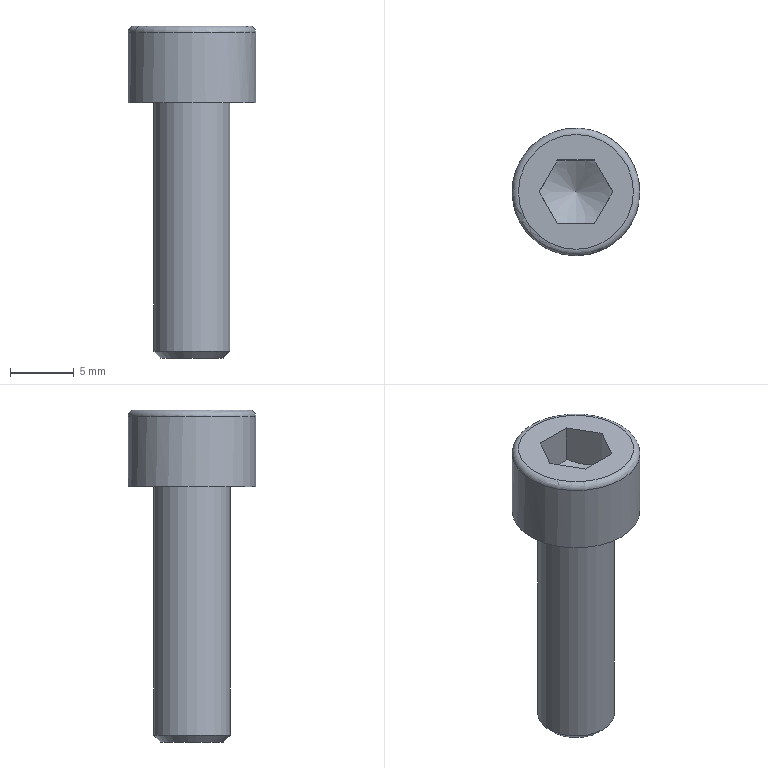Part | STEP file | 1_19 | 1 solid | 14 faces | box 10 x 10 x 26 mm | volume 953.385 mm3 | plane 9 | cylinder 2 | cone 2 | torus 1 | commonest cylinder face diameters 6 x1 10 x1
STEP:
#1=CARTESIAN_POINT('',(0.,0.,0.));
#2=DIRECTION('',(0.,0.,1.));
#3=DIRECTION('',(1.,0.,0.));
#4=AXIS2_PLACEMENT_3D('',#1,#2,#3);
#5=CARTESIAN_POINT('',(0.,-5.,0.));
#6=VERTEX_POINT('',#5);
#7=CARTESIAN_POINT('',(0.,0.,0.));
#8=DIRECTION('',(0.,0.,1.));
#9=DIRECTION('',(1.,0.,0.));
#10=AXIS2_PLACEMENT_3D('',#7,#8,#9);
#11=CIRCLE('',#10,5.);
#12=CARTESIAN_POINT('',(0.,0.,2.75));
#13=DIRECTION('',(0.,0.,1.));
#14=DIRECTION('',(0.,-1.,0.));
#15=AXIS2_PLACEMENT_3D('',#12,#13,#14);
#16=CYLINDRICAL_SURFACE('',#15,5.);
#17=CARTESIAN_POINT('',(-4.712,-2.75));
#18=DIRECTION('',(1.,0.));
#19=VECTOR('',#18,1.);
#20=LINE('',#17,#19);
#21=(GEOMETRIC_REPRESENTATION_CONTEXT(2)PARAMETRIC_REPRESENTATION_CONTEXT()REPRESENTATION_CONTEXT('',''));
#22=DEFINITIONAL_REPRESENTATION('',(#20),#21);
#23=PCURVE('',#16,#22);
#24=CARTESIAN_POINT('',(0.,2.5,0.));
#25=DIRECTION('',(0.,0.,-1.));
#26=DIRECTION('',(-1.,0.,0.));
#27=AXIS2_PLACEMENT_3D('',#24,#25,#26);
#28=PLANE('',#27);
#29=CARTESIAN_POINT('',(-5.,-2.5));
#30=CARTESIAN_POINT('',(-5.,6.16));
#31=CARTESIAN_POINT('',(2.5,1.83));
#32=CARTESIAN_POINT('',(10.,-2.5));
#33=CARTESIAN_POINT('',(2.5,-6.83));
#34=CARTESIAN_POINT('',(-5.,-11.16));
#35=CARTESIAN_POINT('',(-5.,-2.5));
#36=(BOUNDED_CURVE()B_SPLINE_CURVE(2,(#29,#30,#31,#32,#33,#34,#35),.UNSPECIFIED.,.T.,.F.)B_SPLINE_CURVE_WITH_KNOTS((1,2,2,2,2,1),(-2.094,0.,2.094,4.189,6.283,8.378),.UNSPECIFIED.)CURVE()GEOMETRIC_REPRESENTATION_ITEM()RATIONAL_B_SPLINE_CURVE((1.,0.5,1.,0.5,1.,0.5,1.))REPRESENTATION_ITEM(''));
#37=(GEOMETRIC_REPRESENTATION_CONTEXT(2)PARAMETRIC_REPRESENTATION_CONTEXT()REPRESENTATION_CONTEXT('',''));
#38=DEFINITIONAL_REPRESENTATION('',(#36),#37);
#39=PCURVE('',#28,#38);
#40=SURFACE_CURVE('',#11,(#23,#39),.PCURVE_S1.);
#41=EDGE_CURVE('',#6,#6,#40,.T.);
#42=ORIENTED_EDGE('',*,*,#41,.T.);
#43=CARTESIAN_POINT('',(0.,-5.,5.5));
#44=VERTEX_POINT('',#43);
#45=CARTESIAN_POINT('',(0.,-5.,0.));
#46=CARTESIAN_POINT('',(0.,-5.,5.5));
#47=B_SPLINE_CURVE_WITH_KNOTS('',1,(#45,#46),.UNSPECIFIED.,.F.,.F.,(2,2),(-2.75,2.75),.PIECEWISE_BEZIER_KNOTS.);
#48=CARTESIAN_POINT('',(6.283,0.));
#49=DIRECTION('',(0.,1.));
#50=VECTOR('',#49,1.);
#51=LINE('',#48,#50);
#52=(GEOMETRIC_REPRESENTATION_CONTEXT(2)PARAMETRIC_REPRESENTATION_CONTEXT()REPRESENTATION_CONTEXT('',''));
#53=DEFINITIONAL_REPRESENTATION('',(#51),#52);
#54=PCURVE('',#16,#53);
#55=CARTESIAN_POINT('',(0.,0.));
#56=DIRECTION('',(0.,1.));
#57=VECTOR('',#56,1.);
#58=LINE('',#55,#57);
#59=(GEOMETRIC_REPRESENTATION_CONTEXT(2)PARAMETRIC_REPRESENTATION_CONTEXT()REPRESENTATION_CONTEXT('',''));
#60=DEFINITIONAL_REPRESENTATION('',(#58),#59);
#61=PCURVE('',#16,#60);
#62=SEAM_CURVE('',#47,(#54,#61),.PCURVE_S1.);
#63=EDGE_CURVE('',#6,#44,#62,.T.);
#64=ORIENTED_EDGE('',*,*,#63,.T.);
#65=CARTESIAN_POINT('',(5.,0.,5.5));
#66=VERTEX_POINT('',#65);
#67=CARTESIAN_POINT('',(0.,0.,5.5));
#68=DIRECTION('',(0.,0.,1.));
#69=DIRECTION('',(1.,0.,0.));
#70=AXIS2_PLACEMENT_3D('',#67,#68,#69);
#71=CIRCLE('',#70,5.);
#72=CARTESIAN_POINT('',(1.571,2.75));
#73=DIRECTION('',(1.,0.));
#74=VECTOR('',#73,1.);
#75=LINE('',#72,#74);
#76=(GEOMETRIC_REPRESENTATION_CONTEXT(2)PARAMETRIC_REPRESENTATION_CONTEXT()REPRESENTATION_CONTEXT('',''));
#77=DEFINITIONAL_REPRESENTATION('',(#75),#76);
#78=PCURVE('',#16,#77);
#79=CARTESIAN_POINT('',(0.,0.,5.5));
#80=DIRECTION('',(0.,0.,-1.));
#81=DIRECTION('',(-1.,0.,0.));
#82=AXIS2_PLACEMENT_3D('',#79,#80,#81);
#83=TOROIDAL_SURFACE('',#82,4.5,0.5);
#84=CARTESIAN_POINT('',(9.425,6.283));
#85=DIRECTION('',(-1.,0.));
#86=VECTOR('',#85,1.);
#87=LINE('',#84,#86);
#88=(GEOMETRIC_REPRESENTATION_CONTEXT(2)PARAMETRIC_REPRESENTATION_CONTEXT()REPRESENTATION_CONTEXT('',''));
#89=DEFINITIONAL_REPRESENTATION('',(#87),#88);
#90=PCURVE('',#83,#89);
#91=SURFACE_CURVE('',#71,(#78,#90),.PCURVE_S1.);
#92=EDGE_CURVE('',#66,#44,#91,.T.);
#93=ORIENTED_EDGE('',*,*,#92,.F.);
#94=CARTESIAN_POINT('',(0.,0.,5.5));
#95=DIRECTION('',(0.,0.,1.));
#96=DIRECTION('',(1.,0.,0.));
#97=AXIS2_PLACEMENT_3D('',#94,#95,#96);
#98=CIRCLE('',#97,5.);
#99=CARTESIAN_POINT('',(-4.712,2.75));
#100=DIRECTION('',(1.,0.));
#101=VECTOR('',#100,1.);
#102=LINE('',#99,#101);
#103=(GEOMETRIC_REPRESENTATION_CONTEXT(2)PARAMETRIC_REPRESENTATION_CONTEXT()REPRESENTATION_CONTEXT('',''));
#104=DEFINITIONAL_REPRESENTATION('',(#102),#103);
#105=PCURVE('',#16,#104);
#106=CARTESIAN_POINT('',(15.708,6.283));
#107=DIRECTION('',(-1.,0.));
#108=VECTOR('',#107,1.);
#109=LINE('',#106,#108);
#110=(GEOMETRIC_REPRESENTATION_CONTEXT(2)PARAMETRIC_REPRESENTATION_CONTEXT()REPRESENTATION_CONTEXT('',''));
#111=DEFINITIONAL_REPRESENTATION('',(#109),#110);
#112=PCURVE('',#83,#111);
#113=SURFACE_CURVE('',#98,(#105,#112),.PCURVE_S1.);
#114=EDGE_CURVE('',#44,#66,#113,.T.);
#115=ORIENTED_EDGE('',*,*,#114,.F.);
#116=ORIENTED_EDGE('',*,*,#63,.F.);
#117=EDGE_LOOP('',(#42,#64,#93,#115,#116));
#118=FACE_BOUND('',#117,.T.);
#119=ADVANCED_FACE('',(#118),#16,.T.);
#120=ORIENTED_EDGE('',*,*,#92,.T.);
#121=CARTESIAN_POINT('',(0.,-4.5,6.));
#122=VERTEX_POINT('',#121);
#123=CARTESIAN_POINT('',(0.,-4.5,6.));
#124=CARTESIAN_POINT('',(0.,-4.634,6.));
#125=CARTESIAN_POINT('',(0.,-4.764,5.957));
#126=CARTESIAN_POINT('',(0.,-4.876,5.876));
#127=CARTESIAN_POINT('',(0.,-4.957,5.764));
#128=CARTESIAN_POINT('',(0.,-5.,5.634));
#129=CARTESIAN_POINT('',(0.,-5.,5.5));
#130=(BOUNDED_CURVE()B_SPLINE_CURVE(6,(#123,#124,#125,#126,#127,#128,#129),.UNSPECIFIED.,.F.,.F.)B_SPLINE_CURVE_WITH_KNOTS((7,7),(-1.571,0.),.PIECEWISE_BEZIER_KNOTS.)CURVE()GEOMETRIC_REPRESENTATION_ITEM()RATIONAL_B_SPLINE_CURVE((1.031,1.01,0.9979,0.994,0.9979,1.01,1.031))REPRESENTATION_ITEM(''));
#131=CARTESIAN_POINT('',(4.712,6.283));
#132=DIRECTION('',(0.,1.));
#133=VECTOR('',#132,1.);
#134=LINE('',#131,#133);
#135=(GEOMETRIC_REPRESENTATION_CONTEXT(2)PARAMETRIC_REPRESENTATION_CONTEXT()REPRESENTATION_CONTEXT('',''));
#136=DEFINITIONAL_REPRESENTATION('',(#134),#135);
#137=PCURVE('',#83,#136);
#138=CARTESIAN_POINT('',(10.996,6.283));
#139=DIRECTION('',(0.,1.));
#140=VECTOR('',#139,1.);
#141=LINE('',#138,#140);
#142=(GEOMETRIC_REPRESENTATION_CONTEXT(2)PARAMETRIC_REPRESENTATION_CONTEXT()REPRESENTATION_CONTEXT('',''));
#143=DEFINITIONAL_REPRESENTATION('',(#141),#142);
#144=PCURVE('',#83,#143);
#145=SEAM_CURVE('',#130,(#137,#144),.PCURVE_S1.);
#146=EDGE_CURVE('',#122,#44,#145,.T.);
#147=ORIENTED_EDGE('',*,*,#146,.F.);
#148=CARTESIAN_POINT('',(0.,4.5,6.));
#149=VERTEX_POINT('',#148);
#150=CARTESIAN_POINT('',(0.,0.,6.));
#151=DIRECTION('',(0.,0.,-1.));
#152=DIRECTION('',(1.,0.,0.));
#153=AXIS2_PLACEMENT_3D('',#150,#151,#152);
#154=CIRCLE('',#153,4.5);
#155=CARTESIAN_POINT('',(3.142,4.712));
#156=DIRECTION('',(1.,0.));
#157=VECTOR('',#156,1.);
#158=LINE('',#155,#157);
#159=(GEOMETRIC_REPRESENTATION_CONTEXT(2)PARAMETRIC_REPRESENTATION_CONTEXT()REPRESENTATION_CONTEXT('',''));
#160=DEFINITIONAL_REPRESENTATION('',(#158),#159);
#161=PCURVE('',#83,#160);
#162=CARTESIAN_POINT('',(0.,2.25,6.));
#163=DIRECTION('',(0.,0.,1.));
#164=DIRECTION('',(1.,0.,0.));
#165=AXIS2_PLACEMENT_3D('',#162,#163,#164);
#166=PLANE('',#165);
#167=CARTESIAN_POINT('',(4.5,-2.25));
#168=CARTESIAN_POINT('',(4.5,-10.044));
#169=CARTESIAN_POINT('',(-2.25,-6.147));
#170=CARTESIAN_POINT('',(-9.,-2.25));
#171=CARTESIAN_POINT('',(-2.25,1.647));
#172=CARTESIAN_POINT('',(4.5,5.544));
#173=CARTESIAN_POINT('',(4.5,-2.25));
#174=(BOUNDED_CURVE()B_SPLINE_CURVE(2,(#167,#168,#169,#170,#171,#172,#173),.UNSPECIFIED.,.T.,.F.)B_SPLINE_CURVE_WITH_KNOTS((1,2,2,2,2,1),(-2.094,0.,2.094,4.189,6.283,8.378),.UNSPECIFIED.)CURVE()GEOMETRIC_REPRESENTATION_ITEM()RATIONAL_B_SPLINE_CURVE((1.,0.5,1.,0.5,1.,0.5,1.))REPRESENTATION_ITEM(''));
#175=(GEOMETRIC_REPRESENTATION_CONTEXT(2)PARAMETRIC_REPRESENTATION_CONTEXT()REPRESENTATION_CONTEXT('',''));
#176=DEFINITIONAL_REPRESENTATION('',(#174),#175);
#177=PCURVE('',#166,#176);
#178=SURFACE_CURVE('',#154,(#161,#177),.PCURVE_S1.);
#179=EDGE_CURVE('',#122,#149,#178,.T.);
#180=ORIENTED_EDGE('',*,*,#179,.T.);
#181=CARTESIAN_POINT('',(0.,0.,6.));
#182=DIRECTION('',(0.,0.,-1.));
#183=DIRECTION('',(1.,0.,0.));
#184=AXIS2_PLACEMENT_3D('',#181,#182,#183);
#185=CIRCLE('',#184,4.5);
#186=CARTESIAN_POINT('',(3.142,4.712));
#187=DIRECTION('',(1.,0.));
#188=VECTOR('',#187,1.);
#189=LINE('',#186,#188);
#190=(GEOMETRIC_REPRESENTATION_CONTEXT(2)PARAMETRIC_REPRESENTATION_CONTEXT()REPRESENTATION_CONTEXT('',''));
#191=DEFINITIONAL_REPRESENTATION('',(#189),#190);
#192=PCURVE('',#83,#191);
#193=CARTESIAN_POINT('',(4.5,-2.25));
#194=CARTESIAN_POINT('',(4.5,-10.044));
#195=CARTESIAN_POINT('',(-2.25,-6.147));
#196=CARTESIAN_POINT('',(-9.,-2.25));
#197=CARTESIAN_POINT('',(-2.25,1.647));
#198=CARTESIAN_POINT('',(4.5,5.544));
#199=CARTESIAN_POINT('',(4.5,-2.25));
#200=(BOUNDED_CURVE()B_SPLINE_CURVE(2,(#193,#194,#195,#196,#197,#198,#199),.UNSPECIFIED.,.T.,.F.)B_SPLINE_CURVE_WITH_KNOTS((1,2,2,2,2,1),(-2.094,0.,2.094,4.189,6.283,8.378),.UNSPECIFIED.)CURVE()GEOMETRIC_REPRESENTATION_ITEM()RATIONAL_B_SPLINE_CURVE((1.,0.5,1.,0.5,1.,0.5,1.))REPRESENTATION_ITEM(''));
#201=(GEOMETRIC_REPRESENTATION_CONTEXT(2)PARAMETRIC_REPRESENTATION_CONTEXT()REPRESENTATION_CONTEXT('',''));
#202=DEFINITIONAL_REPRESENTATION('',(#200),#201);
#203=PCURVE('',#166,#202);
#204=SURFACE_CURVE('',#185,(#192,#203),.PCURVE_S1.);
#205=EDGE_CURVE('',#149,#122,#204,.T.);
#206=ORIENTED_EDGE('',*,*,#205,.T.);
#207=ORIENTED_EDGE('',*,*,#146,.T.);
#208=ORIENTED_EDGE('',*,*,#114,.T.);
#209=EDGE_LOOP('',(#120,#147,#180,#206,#207,#208));
#210=FACE_BOUND('',#209,.T.);
#211=ADVANCED_FACE('',(#210),#83,.T.);
#212=ORIENTED_EDGE('',*,*,#41,.F.);
#213=EDGE_LOOP('',(#212));
#214=FACE_BOUND('',#213,.T.);
#215=CARTESIAN_POINT('',(0.,-3.,0.));
#216=VERTEX_POINT('',#215);
#217=CARTESIAN_POINT('',(0.,0.,0.));
#218=DIRECTION('',(0.,0.,1.));
#219=DIRECTION('',(0.,1.,0.));
#220=AXIS2_PLACEMENT_3D('',#217,#218,#219);
#221=CIRCLE('',#220,3.);
#222=CARTESIAN_POINT('',(0.,0.5));
#223=CARTESIAN_POINT('',(5.196,0.5));
#224=CARTESIAN_POINT('',(2.598,-4.));
#225=CARTESIAN_POINT('',(0.,-8.5));
#226=CARTESIAN_POINT('',(-2.598,-4.));
#227=CARTESIAN_POINT('',(-5.196,0.5));
#228=CARTESIAN_POINT('',(0.,0.5));
#229=(BOUNDED_CURVE()B_SPLINE_CURVE(2,(#222,#223,#224,#225,#226,#227,#228),.UNSPECIFIED.,.T.,.F.)B_SPLINE_CURVE_WITH_KNOTS((1,2,2,2,2,1),(-2.094,0.,2.094,4.189,6.283,8.378),.UNSPECIFIED.)CURVE()GEOMETRIC_REPRESENTATION_ITEM()RATIONAL_B_SPLINE_CURVE((1.,0.5,1.,0.5,1.,0.5,1.))REPRESENTATION_ITEM(''));
#230=(GEOMETRIC_REPRESENTATION_CONTEXT(2)PARAMETRIC_REPRESENTATION_CONTEXT()REPRESENTATION_CONTEXT('',''));
#231=DEFINITIONAL_REPRESENTATION('',(#229),#230);
#232=PCURVE('',#28,#231);
#233=CARTESIAN_POINT('',(0.,0.,-9.229));
#234=DIRECTION('',(0.,0.,1.));
#235=DIRECTION('',(0.,-1.,0.));
#236=AXIS2_PLACEMENT_3D('',#233,#234,#235);
#237=CYLINDRICAL_SURFACE('',#236,3.);
#238=CARTESIAN_POINT('',(-3.142,9.229));
#239=DIRECTION('',(1.,0.));
#240=VECTOR('',#239,1.);
#241=LINE('',#238,#240);
#242=(GEOMETRIC_REPRESENTATION_CONTEXT(2)PARAMETRIC_REPRESENTATION_CONTEXT()REPRESENTATION_CONTEXT('',''));
#243=DEFINITIONAL_REPRESENTATION('',(#241),#242);
#244=PCURVE('',#237,#243);
#245=SURFACE_CURVE('',#221,(#232,#244),.PCURVE_S1.);
#246=EDGE_CURVE('',#216,#216,#245,.T.);
#247=ORIENTED_EDGE('',*,*,#246,.T.);
#248=EDGE_LOOP('',(#247));
#249=FACE_BOUND('',#248,.T.);
#250=ADVANCED_FACE('',(#214,#249),#28,.T.);
#251=ORIENTED_EDGE('',*,*,#205,.F.);
#252=ORIENTED_EDGE('',*,*,#179,.F.);
#253=EDGE_LOOP('',(#251,#252));
#254=FACE_BOUND('',#253,.T.);
#255=CARTESIAN_POINT('',(-1.443,-2.5,6.));
#256=VERTEX_POINT('',#255);
#257=CARTESIAN_POINT('',(-2.887,0.,6.));
#258=VERTEX_POINT('',#257);
#259=CARTESIAN_POINT('',(-1.443,-2.5,6.));
#260=DIRECTION('',(-0.5,0.866,0.));
#261=VECTOR('',#260,1.);
#262=LINE('',#259,#261);
#263=CARTESIAN_POINT('',(-1.443,-4.75));
#264=DIRECTION('',(-0.5,0.866));
#265=VECTOR('',#264,1.);
#266=LINE('',#263,#265);
#267=(GEOMETRIC_REPRESENTATION_CONTEXT(2)PARAMETRIC_REPRESENTATION_CONTEXT()REPRESENTATION_CONTEXT('',''));
#268=DEFINITIONAL_REPRESENTATION('',(#266),#267);
#269=PCURVE('',#166,#268);
#270=CARTESIAN_POINT('',(-2.887,0.,6.));
#271=DIRECTION('',(-0.866,-0.5,0.));
#272=DIRECTION('',(0.,0.,1.));
#273=AXIS2_PLACEMENT_3D('',#270,#271,#272);
#274=PLANE('',#273);
#275=CARTESIAN_POINT('',(0.,-2.887));
#276=DIRECTION('',(0.,1.));
#277=VECTOR('',#276,1.);
#278=LINE('',#275,#277);
#279=(GEOMETRIC_REPRESENTATION_CONTEXT(2)PARAMETRIC_REPRESENTATION_CONTEXT()REPRESENTATION_CONTEXT('',''));
#280=DEFINITIONAL_REPRESENTATION('',(#278),#279);
#281=PCURVE('',#274,#280);
#282=SURFACE_CURVE('',#262,(#269,#281),.PCURVE_S1.);
#283=EDGE_CURVE('',#256,#258,#282,.T.);
#284=ORIENTED_EDGE('',*,*,#283,.T.);
#285=CARTESIAN_POINT('',(-1.443,2.5,6.));
#286=VERTEX_POINT('',#285);
#287=CARTESIAN_POINT('',(-2.887,0.,6.));
#288=DIRECTION('',(0.5,0.866,0.));
#289=VECTOR('',#288,1.);
#290=LINE('',#287,#289);
#291=CARTESIAN_POINT('',(-2.887,-2.25));
#292=DIRECTION('',(0.5,0.866));
#293=VECTOR('',#292,1.);
#294=LINE('',#291,#293);
#295=(GEOMETRIC_REPRESENTATION_CONTEXT(2)PARAMETRIC_REPRESENTATION_CONTEXT()REPRESENTATION_CONTEXT('',''));
#296=DEFINITIONAL_REPRESENTATION('',(#294),#295);
#297=PCURVE('',#166,#296);
#298=CARTESIAN_POINT('',(-1.443,2.5,6.));
#299=DIRECTION('',(-0.866,0.5,0.));
#300=DIRECTION('',(0.,0.,1.));
#301=AXIS2_PLACEMENT_3D('',#298,#299,#300);
#302=PLANE('',#301);
#303=CARTESIAN_POINT('',(0.,-2.887));
#304=DIRECTION('',(0.,1.));
#305=VECTOR('',#304,1.);
#306=LINE('',#303,#305);
#307=(GEOMETRIC_REPRESENTATION_CONTEXT(2)PARAMETRIC_REPRESENTATION_CONTEXT()REPRESENTATION_CONTEXT('',''));
#308=DEFINITIONAL_REPRESENTATION('',(#306),#307);
#309=PCURVE('',#302,#308);
#310=SURFACE_CURVE('',#290,(#297,#309),.PCURVE_S1.);
#311=EDGE_CURVE('',#258,#286,#310,.T.);
#312=ORIENTED_EDGE('',*,*,#311,.T.);
#313=CARTESIAN_POINT('',(1.443,2.5,6.));
#314=VERTEX_POINT('',#313);
#315=CARTESIAN_POINT('',(-1.443,2.5,6.));
#316=DIRECTION('',(1.,0.,0.));
#317=VECTOR('',#316,1.);
#318=LINE('',#315,#317);
#319=CARTESIAN_POINT('',(-1.443,0.25));
#320=DIRECTION('',(1.,0.));
#321=VECTOR('',#320,1.);
#322=LINE('',#319,#321);
#323=(GEOMETRIC_REPRESENTATION_CONTEXT(2)PARAMETRIC_REPRESENTATION_CONTEXT()REPRESENTATION_CONTEXT('',''));
#324=DEFINITIONAL_REPRESENTATION('',(#322),#323);
#325=PCURVE('',#166,#324);
#326=CARTESIAN_POINT('',(1.443,2.5,6.));
#327=DIRECTION('',(0.,1.,0.));
#328=DIRECTION('',(0.,0.,1.));
#329=AXIS2_PLACEMENT_3D('',#326,#327,#328);
#330=PLANE('',#329);
#331=CARTESIAN_POINT('',(0.,-2.887));
#332=DIRECTION('',(0.,1.));
#333=VECTOR('',#332,1.);
#334=LINE('',#331,#333);
#335=(GEOMETRIC_REPRESENTATION_CONTEXT(2)PARAMETRIC_REPRESENTATION_CONTEXT()REPRESENTATION_CONTEXT('',''));
#336=DEFINITIONAL_REPRESENTATION('',(#334),#335);
#337=PCURVE('',#330,#336);
#338=SURFACE_CURVE('',#318,(#325,#337),.PCURVE_S1.);
#339=EDGE_CURVE('',#286,#314,#338,.T.);
#340=ORIENTED_EDGE('',*,*,#339,.T.);
#341=CARTESIAN_POINT('',(2.887,0.,6.));
#342=VERTEX_POINT('',#341);
#343=CARTESIAN_POINT('',(1.443,2.5,6.));
#344=DIRECTION('',(0.5,-0.866,0.));
#345=VECTOR('',#344,1.);
#346=LINE('',#343,#345);
#347=CARTESIAN_POINT('',(1.443,0.25));
#348=DIRECTION('',(0.5,-0.866));
#349=VECTOR('',#348,1.);
#350=LINE('',#347,#349);
#351=(GEOMETRIC_REPRESENTATION_CONTEXT(2)PARAMETRIC_REPRESENTATION_CONTEXT()REPRESENTATION_CONTEXT('',''));
#352=DEFINITIONAL_REPRESENTATION('',(#350),#351);
#353=PCURVE('',#166,#352);
#354=CARTESIAN_POINT('',(2.887,0.,6.));
#355=DIRECTION('',(0.866,0.5,0.));
#356=DIRECTION('',(0.,0.,-1.));
#357=AXIS2_PLACEMENT_3D('',#354,#355,#356);
#358=PLANE('',#357);
#359=CARTESIAN_POINT('',(0.,2.887));
#360=DIRECTION('',(0.,-1.));
#361=VECTOR('',#360,1.);
#362=LINE('',#359,#361);
#363=(GEOMETRIC_REPRESENTATION_CONTEXT(2)PARAMETRIC_REPRESENTATION_CONTEXT()REPRESENTATION_CONTEXT('',''));
#364=DEFINITIONAL_REPRESENTATION('',(#362),#363);
#365=PCURVE('',#358,#364);
#366=SURFACE_CURVE('',#346,(#353,#365),.PCURVE_S1.);
#367=EDGE_CURVE('',#314,#342,#366,.T.);
#368=ORIENTED_EDGE('',*,*,#367,.T.);
#369=CARTESIAN_POINT('',(1.443,-2.5,6.));
#370=VERTEX_POINT('',#369);
#371=CARTESIAN_POINT('',(2.887,0.,6.));
#372=DIRECTION('',(-0.5,-0.866,0.));
#373=VECTOR('',#372,1.);
#374=LINE('',#371,#373);
#375=CARTESIAN_POINT('',(2.887,-2.25));
#376=DIRECTION('',(-0.5,-0.866));
#377=VECTOR('',#376,1.);
#378=LINE('',#375,#377);
#379=(GEOMETRIC_REPRESENTATION_CONTEXT(2)PARAMETRIC_REPRESENTATION_CONTEXT()REPRESENTATION_CONTEXT('',''));
#380=DEFINITIONAL_REPRESENTATION('',(#378),#379);
#381=PCURVE('',#166,#380);
#382=CARTESIAN_POINT('',(1.443,-2.5,6.));
#383=DIRECTION('',(0.866,-0.5,0.));
#384=DIRECTION('',(0.,0.,-1.));
#385=AXIS2_PLACEMENT_3D('',#382,#383,#384);
#386=PLANE('',#385);
#387=CARTESIAN_POINT('',(0.,2.887));
#388=DIRECTION('',(0.,-1.));
#389=VECTOR('',#388,1.);
#390=LINE('',#387,#389);
#391=(GEOMETRIC_REPRESENTATION_CONTEXT(2)PARAMETRIC_REPRESENTATION_CONTEXT()REPRESENTATION_CONTEXT('',''));
#392=DEFINITIONAL_REPRESENTATION('',(#390),#391);
#393=PCURVE('',#386,#392);
#394=SURFACE_CURVE('',#374,(#381,#393),.PCURVE_S1.);
#395=EDGE_CURVE('',#342,#370,#394,.T.);
#396=ORIENTED_EDGE('',*,*,#395,.T.);
#397=CARTESIAN_POINT('',(1.443,-2.5,6.));
#398=DIRECTION('',(-1.,0.,0.));
#399=VECTOR('',#398,1.);
#400=LINE('',#397,#399);
#401=CARTESIAN_POINT('',(1.443,-4.75));
#402=DIRECTION('',(-1.,0.));
#403=VECTOR('',#402,1.);
#404=LINE('',#401,#403);
#405=(GEOMETRIC_REPRESENTATION_CONTEXT(2)PARAMETRIC_REPRESENTATION_CONTEXT()REPRESENTATION_CONTEXT('',''));
#406=DEFINITIONAL_REPRESENTATION('',(#404),#405);
#407=PCURVE('',#166,#406);
#408=CARTESIAN_POINT('',(-1.443,-2.5,6.));
#409=DIRECTION('',(0.,-1.,0.));
#410=DIRECTION('',(0.,0.,-1.));
#411=AXIS2_PLACEMENT_3D('',#408,#409,#410);
#412=PLANE('',#411);
#413=CARTESIAN_POINT('',(0.,2.887));
#414=DIRECTION('',(0.,-1.));
#415=VECTOR('',#414,1.);
#416=LINE('',#413,#415);
#417=(GEOMETRIC_REPRESENTATION_CONTEXT(2)PARAMETRIC_REPRESENTATION_CONTEXT()REPRESENTATION_CONTEXT('',''));
#418=DEFINITIONAL_REPRESENTATION('',(#416),#417);
#419=PCURVE('',#412,#418);
#420=SURFACE_CURVE('',#400,(#407,#419),.PCURVE_S1.);
#421=EDGE_CURVE('',#370,#256,#420,.T.);
#422=ORIENTED_EDGE('',*,*,#421,.T.);
#423=EDGE_LOOP('',(#284,#312,#340,#368,#396,#422));
#424=FACE_BOUND('',#423,.T.);
#425=ADVANCED_FACE('',(#254,#424),#166,.T.);
#426=CARTESIAN_POINT('',(0.,-3.,-19.459));
#427=VERTEX_POINT('',#426);
#428=CARTESIAN_POINT('',(0.,0.,-19.459));
#429=DIRECTION('',(0.,0.,1.));
#430=DIRECTION('',(1.,0.,0.));
#431=AXIS2_PLACEMENT_3D('',#428,#429,#430);
#432=CIRCLE('',#431,3.);
#433=CARTESIAN_POINT('',(-4.712,-10.229));
#434=DIRECTION('',(1.,0.));
#435=VECTOR('',#434,1.);
#436=LINE('',#433,#435);
#437=(GEOMETRIC_REPRESENTATION_CONTEXT(2)PARAMETRIC_REPRESENTATION_CONTEXT()REPRESENTATION_CONTEXT('',''));
#438=DEFINITIONAL_REPRESENTATION('',(#436),#437);
#439=PCURVE('',#237,#438);
#440=CARTESIAN_POINT('',(0.,0.,-19.729));
#441=DIRECTION('',(0.,0.,1.));
#442=DIRECTION('',(0.,-1.,0.));
#443=AXIS2_PLACEMENT_3D('',#440,#441,#442);
#444=CONICAL_SURFACE('',#443,2.729,0.7854);
#445=CARTESIAN_POINT('',(-4.712,0.2706));
#446=DIRECTION('',(1.,0.));
#447=VECTOR('',#446,1.);
#448=LINE('',#445,#447);
#449=(GEOMETRIC_REPRESENTATION_CONTEXT(2)PARAMETRIC_REPRESENTATION_CONTEXT()REPRESENTATION_CONTEXT('',''));
#450=DEFINITIONAL_REPRESENTATION('',(#448),#449);
#451=PCURVE('',#444,#450);
#452=SURFACE_CURVE('',#432,(#439,#451),.PCURVE_S1.);
#453=EDGE_CURVE('',#427,#427,#452,.T.);
#454=ORIENTED_EDGE('',*,*,#453,.T.);
#455=CARTESIAN_POINT('',(0.,-3.,-19.459));
#456=CARTESIAN_POINT('',(0.,-3.,0.));
#457=B_SPLINE_CURVE_WITH_KNOTS('',1,(#455,#456),.UNSPECIFIED.,.F.,.F.,(2,2),(-10.229,9.229),.PIECEWISE_BEZIER_KNOTS.);
#458=CARTESIAN_POINT('',(6.283,0.));
#459=DIRECTION('',(0.,1.));
#460=VECTOR('',#459,1.);
#461=LINE('',#458,#460);
#462=(GEOMETRIC_REPRESENTATION_CONTEXT(2)PARAMETRIC_REPRESENTATION_CONTEXT()REPRESENTATION_CONTEXT('',''));
#463=DEFINITIONAL_REPRESENTATION('',(#461),#462);
#464=PCURVE('',#237,#463);
#465=CARTESIAN_POINT('',(0.,0.));
#466=DIRECTION('',(0.,1.));
#467=VECTOR('',#466,1.);
#468=LINE('',#465,#467);
#469=(GEOMETRIC_REPRESENTATION_CONTEXT(2)PARAMETRIC_REPRESENTATION_CONTEXT()REPRESENTATION_CONTEXT('',''));
#470=DEFINITIONAL_REPRESENTATION('',(#468),#469);
#471=PCURVE('',#237,#470);
#472=SEAM_CURVE('',#457,(#464,#471),.PCURVE_S1.);
#473=EDGE_CURVE('',#427,#216,#472,.T.);
#474=ORIENTED_EDGE('',*,*,#473,.T.);
#475=ORIENTED_EDGE('',*,*,#246,.F.);
#476=ORIENTED_EDGE('',*,*,#473,.F.);
#477=EDGE_LOOP('',(#454,#474,#475,#476));
#478=FACE_BOUND('',#477,.T.);
#479=ADVANCED_FACE('',(#478),#237,.T.);
#480=CARTESIAN_POINT('',(-1.443,-2.5,3.));
#481=VERTEX_POINT('',#480);
#482=CARTESIAN_POINT('',(-2.887,0.,3.));
#483=VERTEX_POINT('',#482);
#484=CARTESIAN_POINT('',(2.581,-9.47,7.));
#485=CARTESIAN_POINT('',(-2.165,-1.25,1.701));
#486=CARTESIAN_POINT('',(-6.911,6.97,7.));
#487=(BOUNDED_CURVE()B_SPLINE_CURVE(2,(#484,#485,#486),.UNSPECIFIED.,.F.,.F.)B_SPLINE_CURVE_WITH_KNOTS((3,3),(0.,2.078),.PIECEWISE_BEZIER_KNOTS.)CURVE()GEOMETRIC_REPRESENTATION_ITEM()RATIONAL_B_SPLINE_CURVE((1.,3.926,1.))REPRESENTATION_ITEM(''));
#488=CARTESIAN_POINT('',(1.,-10.935));
#489=CARTESIAN_POINT('',(-4.299,-1.443));
#490=CARTESIAN_POINT('',(1.,8.048));
#491=(BOUNDED_CURVE()B_SPLINE_CURVE(2,(#488,#489,#490),.UNSPECIFIED.,.F.,.F.)B_SPLINE_CURVE_WITH_KNOTS((3,3),(0.,2.078),.PIECEWISE_BEZIER_KNOTS.)CURVE()GEOMETRIC_REPRESENTATION_ITEM()RATIONAL_B_SPLINE_CURVE((1.,3.926,1.))REPRESENTATION_ITEM(''));
#492=(GEOMETRIC_REPRESENTATION_CONTEXT(2)PARAMETRIC_REPRESENTATION_CONTEXT()REPRESENTATION_CONTEXT('',''));
#493=DEFINITIONAL_REPRESENTATION('',(#491),#492);
#494=PCURVE('',#274,#493);
#495=CARTESIAN_POINT('',(0.,0.,2.167));
#496=DIRECTION('',(0.,0.,1.));
#497=DIRECTION('',(0.,1.,0.));
#498=AXIS2_PLACEMENT_3D('',#495,#496,#497);
#499=CONICAL_SURFACE('',#498,1.443,1.047);
#500=CARTESIAN_POINT('',(2.618,0.8333));
#501=CARTESIAN_POINT('',(2.603,0.8188));
#502=CARTESIAN_POINT('',(2.572,0.7913));
#503=CARTESIAN_POINT('',(2.526,0.755));
#504=CARTESIAN_POINT('',(2.479,0.7233));
#505=CARTESIAN_POINT('',(2.432,0.6958));
#506=CARTESIAN_POINT('',(2.385,0.6724));
#507=CARTESIAN_POINT('',(2.337,0.6529));
#508=CARTESIAN_POINT('',(2.289,0.6371));
#509=CARTESIAN_POINT('',(2.24,0.625));
#510=CARTESIAN_POINT('',(2.192,0.6163));
#511=CARTESIAN_POINT('',(2.143,0.6112));
#512=CARTESIAN_POINT('',(2.094,0.6095));
#513=CARTESIAN_POINT('',(2.046,0.6112));
#514=CARTESIAN_POINT('',(1.997,0.6163));
#515=CARTESIAN_POINT('',(1.948,0.625));
#516=CARTESIAN_POINT('',(1.9,0.6371));
#517=CARTESIAN_POINT('',(1.852,0.6529));
#518=CARTESIAN_POINT('',(1.804,0.6724));
#519=CARTESIAN_POINT('',(1.757,0.6958));
#520=CARTESIAN_POINT('',(1.709,0.7233));
#521=CARTESIAN_POINT('',(1.663,0.755));
#522=CARTESIAN_POINT('',(1.616,0.7913));
#523=CARTESIAN_POINT('',(1.586,0.8188));
#524=CARTESIAN_POINT('',(1.571,0.8333));
#525=B_SPLINE_CURVE_WITH_KNOTS('',3,(#500,#501,#502,#503,#504,#505,#506,#507,#508,#509,#510,#511,#512,#513,#514,#515,#516,#517,#518,#519,#520,#521,#522,#523,#524),.UNSPECIFIED.,.F.,.F.,(4,1,1,1,1,1,1,1,1,1,1,1,1,1,1,1,1,1,1,1,1,1,4),(0.6777,0.7105,0.7433,0.7762,0.809,0.8418,0.8747,0.9075,0.9403,0.9732,1.006,1.039,1.072,1.105,1.137,1.17,1.203,1.236,1.269,1.302,1.334,1.367,1.4),.QUASI_UNIFORM_KNOTS.);
#526=(GEOMETRIC_REPRESENTATION_CONTEXT(2)PARAMETRIC_REPRESENTATION_CONTEXT()REPRESENTATION_CONTEXT('',''));
#527=DEFINITIONAL_REPRESENTATION('',(#525),#526);
#528=PCURVE('',#499,#527);
#529=SURFACE_CURVE('',#487,(#494,#528),.PCURVE_S1.);
#530=EDGE_CURVE('',#481,#483,#529,.T.);
#531=ORIENTED_EDGE('',*,*,#530,.T.);
#532=CARTESIAN_POINT('',(-2.887,0.,6.));
#533=DIRECTION('',(0.,0.,-1.));
#534=VECTOR('',#533,1.);
#535=LINE('',#532,#534);
#536=CARTESIAN_POINT('',(0.,0.));
#537=DIRECTION('',(-1.,0.));
#538=VECTOR('',#537,1.);
#539=LINE('',#536,#538);
#540=(GEOMETRIC_REPRESENTATION_CONTEXT(2)PARAMETRIC_REPRESENTATION_CONTEXT()REPRESENTATION_CONTEXT('',''));
#541=DEFINITIONAL_REPRESENTATION('',(#539),#540);
#542=PCURVE('',#274,#541);
#543=CARTESIAN_POINT('',(0.,-2.887));
#544=DIRECTION('',(-1.,0.));
#545=VECTOR('',#544,1.);
#546=LINE('',#543,#545);
#547=(GEOMETRIC_REPRESENTATION_CONTEXT(2)PARAMETRIC_REPRESENTATION_CONTEXT()REPRESENTATION_CONTEXT('',''));
#548=DEFINITIONAL_REPRESENTATION('',(#546),#547);
#549=PCURVE('',#302,#548);
#550=SURFACE_CURVE('',#535,(#542,#549),.PCURVE_S1.);
#551=EDGE_CURVE('',#258,#483,#550,.T.);
#552=ORIENTED_EDGE('',*,*,#551,.F.);
#553=ORIENTED_EDGE('',*,*,#283,.F.);
#554=CARTESIAN_POINT('',(-1.443,-2.5,6.));
#555=DIRECTION('',(0.,0.,-1.));
#556=VECTOR('',#555,1.);
#557=LINE('',#554,#556);
#558=CARTESIAN_POINT('',(0.,-2.887));
#559=DIRECTION('',(-1.,0.));
#560=VECTOR('',#559,1.);
#561=LINE('',#558,#560);
#562=(GEOMETRIC_REPRESENTATION_CONTEXT(2)PARAMETRIC_REPRESENTATION_CONTEXT()REPRESENTATION_CONTEXT('',''));
#563=DEFINITIONAL_REPRESENTATION('',(#561),#562);
#564=PCURVE('',#274,#563);
#565=CARTESIAN_POINT('',(0.,0.));
#566=DIRECTION('',(1.,0.));
#567=VECTOR('',#566,1.);
#568=LINE('',#565,#567);
#569=(GEOMETRIC_REPRESENTATION_CONTEXT(2)PARAMETRIC_REPRESENTATION_CONTEXT()REPRESENTATION_CONTEXT('',''));
#570=DEFINITIONAL_REPRESENTATION('',(#568),#569);
#571=PCURVE('',#412,#570);
#572=SURFACE_CURVE('',#557,(#564,#571),.PCURVE_S1.);
#573=EDGE_CURVE('',#256,#481,#572,.T.);
#574=ORIENTED_EDGE('',*,*,#573,.T.);
#575=EDGE_LOOP('',(#531,#552,#553,#574));
#576=FACE_BOUND('',#575,.T.);
#577=ADVANCED_FACE('',(#576),#274,.F.);
#578=CARTESIAN_POINT('',(-1.443,2.5,3.));
#579=VERTEX_POINT('',#578);
#580=CARTESIAN_POINT('',(-6.911,-6.97,7.));
#581=CARTESIAN_POINT('',(-2.165,1.25,1.701));
#582=CARTESIAN_POINT('',(2.581,9.47,7.));
#583=(BOUNDED_CURVE()B_SPLINE_CURVE(2,(#580,#581,#582),.UNSPECIFIED.,.F.,.F.)B_SPLINE_CURVE_WITH_KNOTS((3,3),(0.,2.078),.PIECEWISE_BEZIER_KNOTS.)CURVE()GEOMETRIC_REPRESENTATION_ITEM()RATIONAL_B_SPLINE_CURVE((1.,3.926,1.))REPRESENTATION_ITEM(''));
#584=CARTESIAN_POINT('',(1.,-10.935));
#585=CARTESIAN_POINT('',(-4.299,-1.443));
#586=CARTESIAN_POINT('',(1.,8.048));
#587=(BOUNDED_CURVE()B_SPLINE_CURVE(2,(#584,#585,#586),.UNSPECIFIED.,.F.,.F.)B_SPLINE_CURVE_WITH_KNOTS((3,3),(0.,2.078),.PIECEWISE_BEZIER_KNOTS.)CURVE()GEOMETRIC_REPRESENTATION_ITEM()RATIONAL_B_SPLINE_CURVE((1.,3.926,1.))REPRESENTATION_ITEM(''));
#588=(GEOMETRIC_REPRESENTATION_CONTEXT(2)PARAMETRIC_REPRESENTATION_CONTEXT()REPRESENTATION_CONTEXT('',''));
#589=DEFINITIONAL_REPRESENTATION('',(#587),#588);
#590=PCURVE('',#302,#589);
#591=CARTESIAN_POINT('',(1.571,0.8333));
#592=CARTESIAN_POINT('',(1.556,0.8188));
#593=CARTESIAN_POINT('',(1.525,0.7913));
#594=CARTESIAN_POINT('',(1.479,0.755));
#595=CARTESIAN_POINT('',(1.432,0.7233));
#596=CARTESIAN_POINT('',(1.385,0.6958));
#597=CARTESIAN_POINT('',(1.338,0.6724));
#598=CARTESIAN_POINT('',(1.29,0.6529));
#599=CARTESIAN_POINT('',(1.241,0.6371));
#600=CARTESIAN_POINT('',(1.193,0.625));
#601=CARTESIAN_POINT('',(1.145,0.6163));
#602=CARTESIAN_POINT('',(1.096,0.6112));
#603=CARTESIAN_POINT('',(1.047,0.6095));
#604=CARTESIAN_POINT('',(0.9985,0.6112));
#605=CARTESIAN_POINT('',(0.9498,0.6163));
#606=CARTESIAN_POINT('',(0.9013,0.625));
#607=CARTESIAN_POINT('',(0.8529,0.6371));
#608=CARTESIAN_POINT('',(0.8048,0.6529));
#609=CARTESIAN_POINT('',(0.7569,0.6724));
#610=CARTESIAN_POINT('',(0.7094,0.6958));
#611=CARTESIAN_POINT('',(0.6622,0.7233));
#612=CARTESIAN_POINT('',(0.6155,0.755));
#613=CARTESIAN_POINT('',(0.5692,0.7913));
#614=CARTESIAN_POINT('',(0.5388,0.8188));
#615=CARTESIAN_POINT('',(0.5236,0.8333));
#616=B_SPLINE_CURVE_WITH_KNOTS('',3,(#591,#592,#593,#594,#595,#596,#597,#598,#599,#600,#601,#602,#603,#604,#605,#606,#607,#608,#609,#610,#611,#612,#613,#614,#615),.UNSPECIFIED.,.F.,.F.,(4,1,1,1,1,1,1,1,1,1,1,1,1,1,1,1,1,1,1,1,1,1,4),(0.6777,0.7105,0.7433,0.7762,0.809,0.8418,0.8747,0.9075,0.9403,0.9732,1.006,1.039,1.072,1.105,1.137,1.17,1.203,1.236,1.269,1.302,1.334,1.367,1.4),.QUASI_UNIFORM_KNOTS.);
#617=(GEOMETRIC_REPRESENTATION_CONTEXT(2)PARAMETRIC_REPRESENTATION_CONTEXT()REPRESENTATION_CONTEXT('',''));
#618=DEFINITIONAL_REPRESENTATION('',(#616),#617);
#619=PCURVE('',#499,#618);
#620=SURFACE_CURVE('',#583,(#590,#619),.PCURVE_S1.);
#621=EDGE_CURVE('',#483,#579,#620,.T.);
#622=ORIENTED_EDGE('',*,*,#621,.T.);
#623=CARTESIAN_POINT('',(-1.443,2.5,6.));
#624=DIRECTION('',(0.,0.,-1.));
#625=VECTOR('',#624,1.);
#626=LINE('',#623,#625);
#627=CARTESIAN_POINT('',(0.,0.));
#628=DIRECTION('',(-1.,0.));
#629=VECTOR('',#628,1.);
#630=LINE('',#627,#629);
#631=(GEOMETRIC_REPRESENTATION_CONTEXT(2)PARAMETRIC_REPRESENTATION_CONTEXT()REPRESENTATION_CONTEXT('',''));
#632=DEFINITIONAL_REPRESENTATION('',(#630),#631);
#633=PCURVE('',#302,#632);
#634=CARTESIAN_POINT('',(0.,-2.887));
#635=DIRECTION('',(-1.,0.));
#636=VECTOR('',#635,1.);
#637=LINE('',#634,#636);
#638=(GEOMETRIC_REPRESENTATION_CONTEXT(2)PARAMETRIC_REPRESENTATION_CONTEXT()REPRESENTATION_CONTEXT('',''));
#639=DEFINITIONAL_REPRESENTATION('',(#637),#638);
#640=PCURVE('',#330,#639);
#641=SURFACE_CURVE('',#626,(#633,#640),.PCURVE_S1.);
#642=EDGE_CURVE('',#286,#579,#641,.T.);
#643=ORIENTED_EDGE('',*,*,#642,.F.);
#644=ORIENTED_EDGE('',*,*,#311,.F.);
#645=ORIENTED_EDGE('',*,*,#551,.T.);
#646=EDGE_LOOP('',(#622,#643,#644,#645));
#647=FACE_BOUND('',#646,.T.);
#648=ADVANCED_FACE('',(#647),#302,.F.);
#649=CARTESIAN_POINT('',(-0.000000001,2.5,2.777));
#650=VERTEX_POINT('',#649);
#651=CARTESIAN_POINT('',(-1.443,2.5,3.));
#652=CARTESIAN_POINT('',(-1.138,2.5,2.912));
#653=CARTESIAN_POINT('',(-0.8439,2.5,2.844));
#654=CARTESIAN_POINT('',(-0.5591,2.5,2.799));
#655=CARTESIAN_POINT('',(-0.2796,2.5,2.777));
#656=CARTESIAN_POINT('',(-0.000000001,2.5,2.777));
#657=B_SPLINE_CURVE_WITH_KNOTS('',5,(#651,#652,#653,#654,#655,#656),.UNSPECIFIED.,.F.,.F.,(6,6),(0.,2.1),.PIECEWISE_BEZIER_KNOTS.);
#658=CARTESIAN_POINT('',(-3.,-2.887));
#659=CARTESIAN_POINT('',(-3.088,-2.582));
#660=CARTESIAN_POINT('',(-3.156,-2.287));
#661=CARTESIAN_POINT('',(-3.201,-2.002));
#662=CARTESIAN_POINT('',(-3.223,-1.723));
#663=CARTESIAN_POINT('',(-3.223,-1.443));
#664=B_SPLINE_CURVE_WITH_KNOTS('',5,(#658,#659,#660,#661,#662,#663),.UNSPECIFIED.,.F.,.F.,(6,6),(0.,2.1),.PIECEWISE_BEZIER_KNOTS.);
#665=(GEOMETRIC_REPRESENTATION_CONTEXT(2)PARAMETRIC_REPRESENTATION_CONTEXT()REPRESENTATION_CONTEXT('',''));
#666=DEFINITIONAL_REPRESENTATION('',(#664),#665);
#667=PCURVE('',#330,#666);
#668=CARTESIAN_POINT('',(0.5236,0.8333));
#669=CARTESIAN_POINT('',(0.5167,0.8267));
#670=CARTESIAN_POINT('',(0.5027,0.8136));
#671=CARTESIAN_POINT('',(0.4813,0.7949));
#672=CARTESIAN_POINT('',(0.4596,0.777));
#673=CARTESIAN_POINT('',(0.4376,0.76));
#674=CARTESIAN_POINT('',(0.4152,0.7439));
#675=CARTESIAN_POINT('',(0.3926,0.7287));
#676=CARTESIAN_POINT('',(0.3696,0.7144));
#677=CARTESIAN_POINT('',(0.3463,0.701));
#678=CARTESIAN_POINT('',(0.3228,0.6885));
#679=CARTESIAN_POINT('',(0.299,0.6769));
#680=CARTESIAN_POINT('',(0.2749,0.6662));
#681=CARTESIAN_POINT('',(0.2507,0.6564));
#682=CARTESIAN_POINT('',(0.2262,0.6476));
#683=CARTESIAN_POINT('',(0.2015,0.6397));
#684=CARTESIAN_POINT('',(0.1767,0.6327));
#685=CARTESIAN_POINT('',(0.1517,0.6267));
#686=CARTESIAN_POINT('',(0.1266,0.6215));
#687=CARTESIAN_POINT('',(0.1014,0.6173));
#688=CARTESIAN_POINT('',(0.07616,0.6141));
#689=CARTESIAN_POINT('',(0.05081,0.6118));
#690=CARTESIAN_POINT('',(0.02541,0.6104));
#691=CARTESIAN_POINT('',(0.008472,0.61));
#692=CARTESIAN_POINT('',(0.,0.61));
#693=B_SPLINE_CURVE_WITH_KNOTS('',3,(#668,#669,#670,#671,#672,#673,#674,#675,#676,#677,#678,#679,#680,#681,#682,#683,#684,#685,#686,#687,#688,#689,#690,#691,#692),.UNSPECIFIED.,.F.,.F.,(4,1,1,1,1,1,1,1,1,1,1,1,1,1,1,1,1,1,1,1,1,1,4),(0.,0.09546,0.1909,0.2864,0.3818,0.4773,0.5728,0.6682,0.7637,0.8592,0.9546,1.05,1.146,1.241,1.336,1.432,1.527,1.623,1.718,1.814,1.909,2.005,2.1),.QUASI_UNIFORM_KNOTS.);
#694=(GEOMETRIC_REPRESENTATION_CONTEXT(2)PARAMETRIC_REPRESENTATION_CONTEXT()REPRESENTATION_CONTEXT('',''));
#695=DEFINITIONAL_REPRESENTATION('',(#693),#694);
#696=PCURVE('',#499,#695);
#697=SURFACE_CURVE('',#657,(#667,#696),.PCURVE_S1.);
#698=EDGE_CURVE('',#579,#650,#697,.T.);
#699=ORIENTED_EDGE('',*,*,#698,.T.);
#700=CARTESIAN_POINT('',(1.443,2.5,3.));
#701=VERTEX_POINT('',#700);
#702=CARTESIAN_POINT('',(-0.000000001,2.5,2.777));
#703=CARTESIAN_POINT('',(0.2796,2.5,2.777));
#704=CARTESIAN_POINT('',(0.5591,2.5,2.799));
#705=CARTESIAN_POINT('',(0.8439,2.5,2.844));
#706=CARTESIAN_POINT('',(1.138,2.5,2.912));
#707=CARTESIAN_POINT('',(1.443,2.5,3.));
#708=B_SPLINE_CURVE_WITH_KNOTS('',5,(#702,#703,#704,#705,#706,#707),.UNSPECIFIED.,.F.,.F.,(6,6),(0.,2.1),.PIECEWISE_BEZIER_KNOTS.);
#709=CARTESIAN_POINT('',(-3.223,-1.443));
#710=CARTESIAN_POINT('',(-3.223,-1.164));
#711=CARTESIAN_POINT('',(-3.201,-0.8843));
#712=CARTESIAN_POINT('',(-3.156,-0.5995));
#713=CARTESIAN_POINT('',(-3.088,-0.3051));
#714=CARTESIAN_POINT('',(-3.,0.));
#715=B_SPLINE_CURVE_WITH_KNOTS('',5,(#709,#710,#711,#712,#713,#714),.UNSPECIFIED.,.F.,.F.,(6,6),(0.,2.1),.PIECEWISE_BEZIER_KNOTS.);
#716=(GEOMETRIC_REPRESENTATION_CONTEXT(2)PARAMETRIC_REPRESENTATION_CONTEXT()REPRESENTATION_CONTEXT('',''));
#717=DEFINITIONAL_REPRESENTATION('',(#715),#716);
#718=PCURVE('',#330,#717);
#719=CARTESIAN_POINT('',(6.283,0.61));
#720=CARTESIAN_POINT('',(6.275,0.61));
#721=CARTESIAN_POINT('',(6.258,0.6104));
#722=CARTESIAN_POINT('',(6.232,0.6118));
#723=CARTESIAN_POINT('',(6.207,0.6141));
#724=CARTESIAN_POINT('',(6.182,0.6173));
#725=CARTESIAN_POINT('',(6.157,0.6215));
#726=CARTESIAN_POINT('',(6.131,0.6267));
#727=CARTESIAN_POINT('',(6.106,0.6327));
#728=CARTESIAN_POINT('',(6.082,0.6397));
#729=CARTESIAN_POINT('',(6.057,0.6476));
#730=CARTESIAN_POINT('',(6.033,0.6564));
#731=CARTESIAN_POINT('',(6.008,0.6662));
#732=CARTESIAN_POINT('',(5.984,0.6769));
#733=CARTESIAN_POINT('',(5.96,0.6885));
#734=CARTESIAN_POINT('',(5.937,0.701));
#735=CARTESIAN_POINT('',(5.914,0.7144));
#736=CARTESIAN_POINT('',(5.891,0.7287));
#737=CARTESIAN_POINT('',(5.868,0.7439));
#738=CARTESIAN_POINT('',(5.846,0.76));
#739=CARTESIAN_POINT('',(5.824,0.777));
#740=CARTESIAN_POINT('',(5.802,0.7949));
#741=CARTESIAN_POINT('',(5.781,0.8136));
#742=CARTESIAN_POINT('',(5.767,0.8267));
#743=CARTESIAN_POINT('',(5.76,0.8333));
#744=B_SPLINE_CURVE_WITH_KNOTS('',3,(#719,#720,#721,#722,#723,#724,#725,#726,#727,#728,#729,#730,#731,#732,#733,#734,#735,#736,#737,#738,#739,#740,#741,#742,#743),.UNSPECIFIED.,.F.,.F.,(4,1,1,1,1,1,1,1,1,1,1,1,1,1,1,1,1,1,1,1,1,1,4),(0.,0.09546,0.1909,0.2864,0.3818,0.4773,0.5728,0.6682,0.7637,0.8592,0.9546,1.05,1.146,1.241,1.336,1.432,1.527,1.623,1.718,1.814,1.909,2.005,2.1),.QUASI_UNIFORM_KNOTS.);
#745=(GEOMETRIC_REPRESENTATION_CONTEXT(2)PARAMETRIC_REPRESENTATION_CONTEXT()REPRESENTATION_CONTEXT('',''));
#746=DEFINITIONAL_REPRESENTATION('',(#744),#745);
#747=PCURVE('',#499,#746);
#748=SURFACE_CURVE('',#708,(#718,#747),.PCURVE_S1.);
#749=EDGE_CURVE('',#650,#701,#748,.T.);
#750=ORIENTED_EDGE('',*,*,#749,.T.);
#751=CARTESIAN_POINT('',(1.443,2.5,6.));
#752=DIRECTION('',(0.,0.,-1.));
#753=VECTOR('',#752,1.);
#754=LINE('',#751,#753);
#755=CARTESIAN_POINT('',(0.,0.));
#756=DIRECTION('',(-1.,0.));
#757=VECTOR('',#756,1.);
#758=LINE('',#755,#757);
#759=(GEOMETRIC_REPRESENTATION_CONTEXT(2)PARAMETRIC_REPRESENTATION_CONTEXT()REPRESENTATION_CONTEXT('',''));
#760=DEFINITIONAL_REPRESENTATION('',(#758),#759);
#761=PCURVE('',#330,#760);
#762=CARTESIAN_POINT('',(0.,2.887));
#763=DIRECTION('',(1.,0.));
#764=VECTOR('',#763,1.);
#765=LINE('',#762,#764);
#766=(GEOMETRIC_REPRESENTATION_CONTEXT(2)PARAMETRIC_REPRESENTATION_CONTEXT()REPRESENTATION_CONTEXT('',''));
#767=DEFINITIONAL_REPRESENTATION('',(#765),#766);
#768=PCURVE('',#358,#767);
#769=SURFACE_CURVE('',#754,(#761,#768),.PCURVE_S1.);
#770=EDGE_CURVE('',#314,#701,#769,.T.);
#771=ORIENTED_EDGE('',*,*,#770,.F.);
#772=ORIENTED_EDGE('',*,*,#339,.F.);
#773=ORIENTED_EDGE('',*,*,#642,.T.);
#774=EDGE_LOOP('',(#699,#750,#771,#772,#773));
#775=FACE_BOUND('',#774,.T.);
#776=ADVANCED_FACE('',(#775),#330,.F.);
#777=CARTESIAN_POINT('',(2.887,0.,3.));
#778=VERTEX_POINT('',#777);
#779=CARTESIAN_POINT('',(-2.581,9.47,7.));
#780=CARTESIAN_POINT('',(2.165,1.25,1.701));
#781=CARTESIAN_POINT('',(6.911,-6.97,7.));
#782=(BOUNDED_CURVE()B_SPLINE_CURVE(2,(#779,#780,#781),.UNSPECIFIED.,.F.,.F.)B_SPLINE_CURVE_WITH_KNOTS((3,3),(0.,2.078),.PIECEWISE_BEZIER_KNOTS.)CURVE()GEOMETRIC_REPRESENTATION_ITEM()RATIONAL_B_SPLINE_CURVE((1.,3.926,1.))REPRESENTATION_ITEM(''));
#783=CARTESIAN_POINT('',(-1.,10.935));
#784=CARTESIAN_POINT('',(4.299,1.443));
#785=CARTESIAN_POINT('',(-1.,-8.048));
#786=(BOUNDED_CURVE()B_SPLINE_CURVE(2,(#783,#784,#785),.UNSPECIFIED.,.F.,.F.)B_SPLINE_CURVE_WITH_KNOTS((3,3),(0.,2.078),.PIECEWISE_BEZIER_KNOTS.)CURVE()GEOMETRIC_REPRESENTATION_ITEM()RATIONAL_B_SPLINE_CURVE((1.,3.926,1.))REPRESENTATION_ITEM(''));
#787=(GEOMETRIC_REPRESENTATION_CONTEXT(2)PARAMETRIC_REPRESENTATION_CONTEXT()REPRESENTATION_CONTEXT('',''));
#788=DEFINITIONAL_REPRESENTATION('',(#786),#787);
#789=PCURVE('',#358,#788);
#790=CARTESIAN_POINT('',(5.76,0.8333));
#791=CARTESIAN_POINT('',(5.744,0.8188));
#792=CARTESIAN_POINT('',(5.714,0.7913));
#793=CARTESIAN_POINT('',(5.668,0.755));
#794=CARTESIAN_POINT('',(5.621,0.7233));
#795=CARTESIAN_POINT('',(5.574,0.6958));
#796=CARTESIAN_POINT('',(5.526,0.6724));
#797=CARTESIAN_POINT('',(5.478,0.6529));
#798=CARTESIAN_POINT('',(5.43,0.6371));
#799=CARTESIAN_POINT('',(5.382,0.625));
#800=CARTESIAN_POINT('',(5.333,0.6163));
#801=CARTESIAN_POINT('',(5.285,0.6112));
#802=CARTESIAN_POINT('',(5.236,0.6095));
#803=CARTESIAN_POINT('',(5.187,0.6112));
#804=CARTESIAN_POINT('',(5.139,0.6163));
#805=CARTESIAN_POINT('',(5.09,0.625));
#806=CARTESIAN_POINT('',(5.042,0.6371));
#807=CARTESIAN_POINT('',(4.994,0.6529));
#808=CARTESIAN_POINT('',(4.946,0.6724));
#809=CARTESIAN_POINT('',(4.898,0.6958));
#810=CARTESIAN_POINT('',(4.851,0.7233));
#811=CARTESIAN_POINT('',(4.804,0.755));
#812=CARTESIAN_POINT('',(4.758,0.7913));
#813=CARTESIAN_POINT('',(4.728,0.8188));
#814=CARTESIAN_POINT('',(4.712,0.8333));
#815=B_SPLINE_CURVE_WITH_KNOTS('',3,(#790,#791,#792,#793,#794,#795,#796,#797,#798,#799,#800,#801,#802,#803,#804,#805,#806,#807,#808,#809,#810,#811,#812,#813,#814),.UNSPECIFIED.,.F.,.F.,(4,1,1,1,1,1,1,1,1,1,1,1,1,1,1,1,1,1,1,1,1,1,4),(0.6777,0.7105,0.7433,0.7762,0.809,0.8418,0.8747,0.9075,0.9403,0.9732,1.006,1.039,1.072,1.105,1.137,1.17,1.203,1.236,1.269,1.302,1.334,1.367,1.4),.QUASI_UNIFORM_KNOTS.);
#816=(GEOMETRIC_REPRESENTATION_CONTEXT(2)PARAMETRIC_REPRESENTATION_CONTEXT()REPRESENTATION_CONTEXT('',''));
#817=DEFINITIONAL_REPRESENTATION('',(#815),#816);
#818=PCURVE('',#499,#817);
#819=SURFACE_CURVE('',#782,(#789,#818),.PCURVE_S1.);
#820=EDGE_CURVE('',#701,#778,#819,.T.);
#821=ORIENTED_EDGE('',*,*,#820,.T.);
#822=CARTESIAN_POINT('',(2.887,0.,6.));
#823=DIRECTION('',(0.,0.,-1.));
#824=VECTOR('',#823,1.);
#825=LINE('',#822,#824);
#826=CARTESIAN_POINT('',(0.,0.));
#827=DIRECTION('',(1.,0.));
#828=VECTOR('',#827,1.);
#829=LINE('',#826,#828);
#830=(GEOMETRIC_REPRESENTATION_CONTEXT(2)PARAMETRIC_REPRESENTATION_CONTEXT()REPRESENTATION_CONTEXT('',''));
#831=DEFINITIONAL_REPRESENTATION('',(#829),#830);
#832=PCURVE('',#358,#831);
#833=CARTESIAN_POINT('',(0.,2.887));
#834=DIRECTION('',(1.,0.));
#835=VECTOR('',#834,1.);
#836=LINE('',#833,#835);
#837=(GEOMETRIC_REPRESENTATION_CONTEXT(2)PARAMETRIC_REPRESENTATION_CONTEXT()REPRESENTATION_CONTEXT('',''));
#838=DEFINITIONAL_REPRESENTATION('',(#836),#837);
#839=PCURVE('',#386,#838);
#840=SURFACE_CURVE('',#825,(#832,#839),.PCURVE_S1.);
#841=EDGE_CURVE('',#342,#778,#840,.T.);
#842=ORIENTED_EDGE('',*,*,#841,.F.);
#843=ORIENTED_EDGE('',*,*,#367,.F.);
#844=ORIENTED_EDGE('',*,*,#770,.T.);
#845=EDGE_LOOP('',(#821,#842,#843,#844));
#846=FACE_BOUND('',#845,.T.);
#847=ADVANCED_FACE('',(#846),#358,.F.);
#848=CARTESIAN_POINT('',(1.443,-2.5,3.));
#849=VERTEX_POINT('',#848);
#850=CARTESIAN_POINT('',(6.911,6.97,7.));
#851=CARTESIAN_POINT('',(2.165,-1.25,1.701));
#852=CARTESIAN_POINT('',(-2.581,-9.47,7.));
#853=(BOUNDED_CURVE()B_SPLINE_CURVE(2,(#850,#851,#852),.UNSPECIFIED.,.F.,.F.)B_SPLINE_CURVE_WITH_KNOTS((3,3),(0.,2.078),.PIECEWISE_BEZIER_KNOTS.)CURVE()GEOMETRIC_REPRESENTATION_ITEM()RATIONAL_B_SPLINE_CURVE((1.,3.926,1.))REPRESENTATION_ITEM(''));
#854=CARTESIAN_POINT('',(-1.,10.935));
#855=CARTESIAN_POINT('',(4.299,1.443));
#856=CARTESIAN_POINT('',(-1.,-8.048));
#857=(BOUNDED_CURVE()B_SPLINE_CURVE(2,(#854,#855,#856),.UNSPECIFIED.,.F.,.F.)B_SPLINE_CURVE_WITH_KNOTS((3,3),(0.,2.078),.PIECEWISE_BEZIER_KNOTS.)CURVE()GEOMETRIC_REPRESENTATION_ITEM()RATIONAL_B_SPLINE_CURVE((1.,3.926,1.))REPRESENTATION_ITEM(''));
#858=(GEOMETRIC_REPRESENTATION_CONTEXT(2)PARAMETRIC_REPRESENTATION_CONTEXT()REPRESENTATION_CONTEXT('',''));
#859=DEFINITIONAL_REPRESENTATION('',(#857),#858);
#860=PCURVE('',#386,#859);
#861=CARTESIAN_POINT('',(4.712,0.8333));
#862=CARTESIAN_POINT('',(4.697,0.8188));
#863=CARTESIAN_POINT('',(4.667,0.7913));
#864=CARTESIAN_POINT('',(4.621,0.755));
#865=CARTESIAN_POINT('',(4.574,0.7233));
#866=CARTESIAN_POINT('',(4.527,0.6958));
#867=CARTESIAN_POINT('',(4.479,0.6724));
#868=CARTESIAN_POINT('',(4.431,0.6529));
#869=CARTESIAN_POINT('',(4.383,0.6371));
#870=CARTESIAN_POINT('',(4.335,0.625));
#871=CARTESIAN_POINT('',(4.286,0.6163));
#872=CARTESIAN_POINT('',(4.238,0.6112));
#873=CARTESIAN_POINT('',(4.189,0.6095));
#874=CARTESIAN_POINT('',(4.14,0.6112));
#875=CARTESIAN_POINT('',(4.091,0.6163));
#876=CARTESIAN_POINT('',(4.043,0.625));
#877=CARTESIAN_POINT('',(3.994,0.6371));
#878=CARTESIAN_POINT('',(3.946,0.6529));
#879=CARTESIAN_POINT('',(3.898,0.6724));
#880=CARTESIAN_POINT('',(3.851,0.6958));
#881=CARTESIAN_POINT('',(3.804,0.7233));
#882=CARTESIAN_POINT('',(3.757,0.755));
#883=CARTESIAN_POINT('',(3.711,0.7913));
#884=CARTESIAN_POINT('',(3.68,0.8188));
#885=CARTESIAN_POINT('',(3.665,0.8333));
#886=B_SPLINE_CURVE_WITH_KNOTS('',3,(#861,#862,#863,#864,#865,#866,#867,#868,#869,#870,#871,#872,#873,#874,#875,#876,#877,#878,#879,#880,#881,#882,#883,#884,#885),.UNSPECIFIED.,.F.,.F.,(4,1,1,1,1,1,1,1,1,1,1,1,1,1,1,1,1,1,1,1,1,1,4),(0.6777,0.7105,0.7433,0.7762,0.809,0.8418,0.8747,0.9075,0.9403,0.9732,1.006,1.039,1.072,1.105,1.137,1.17,1.203,1.236,1.269,1.302,1.334,1.367,1.4),.QUASI_UNIFORM_KNOTS.);
#887=(GEOMETRIC_REPRESENTATION_CONTEXT(2)PARAMETRIC_REPRESENTATION_CONTEXT()REPRESENTATION_CONTEXT('',''));
#888=DEFINITIONAL_REPRESENTATION('',(#886),#887);
#889=PCURVE('',#499,#888);
#890=SURFACE_CURVE('',#853,(#860,#889),.PCURVE_S1.);
#891=EDGE_CURVE('',#778,#849,#890,.T.);
#892=ORIENTED_EDGE('',*,*,#891,.T.);
#893=CARTESIAN_POINT('',(1.443,-2.5,6.));
#894=DIRECTION('',(0.,0.,-1.));
#895=VECTOR('',#894,1.);
#896=LINE('',#893,#895);
#897=CARTESIAN_POINT('',(0.,0.));
#898=DIRECTION('',(1.,0.));
#899=VECTOR('',#898,1.);
#900=LINE('',#897,#899);
#901=(GEOMETRIC_REPRESENTATION_CONTEXT(2)PARAMETRIC_REPRESENTATION_CONTEXT()REPRESENTATION_CONTEXT('',''));
#902=DEFINITIONAL_REPRESENTATION('',(#900),#901);
#903=PCURVE('',#386,#902);
#904=CARTESIAN_POINT('',(0.,2.887));
#905=DIRECTION('',(1.,0.));
#906=VECTOR('',#905,1.);
#907=LINE('',#904,#906);
#908=(GEOMETRIC_REPRESENTATION_CONTEXT(2)PARAMETRIC_REPRESENTATION_CONTEXT()REPRESENTATION_CONTEXT('',''));
#909=DEFINITIONAL_REPRESENTATION('',(#907),#908);
#910=PCURVE('',#412,#909);
#911=SURFACE_CURVE('',#896,(#903,#910),.PCURVE_S1.);
#912=EDGE_CURVE('',#370,#849,#911,.T.);
#913=ORIENTED_EDGE('',*,*,#912,.F.);
#914=ORIENTED_EDGE('',*,*,#395,.F.);
#915=ORIENTED_EDGE('',*,*,#841,.T.);
#916=EDGE_LOOP('',(#892,#913,#914,#915));
#917=FACE_BOUND('',#916,.T.);
#918=ADVANCED_FACE('',(#917),#386,.F.);
#919=CARTESIAN_POINT('',(0.000000001,-2.5,2.777));
#920=VERTEX_POINT('',#919);
#921=CARTESIAN_POINT('',(1.443,-2.5,3.));
#922=CARTESIAN_POINT('',(1.138,-2.5,2.912));
#923=CARTESIAN_POINT('',(0.8439,-2.5,2.844));
#924=CARTESIAN_POINT('',(0.5591,-2.5,2.799));
#925=CARTESIAN_POINT('',(0.2796,-2.5,2.777));
#926=CARTESIAN_POINT('',(0.000000001,-2.5,2.777));
#927=B_SPLINE_CURVE_WITH_KNOTS('',5,(#921,#922,#923,#924,#925,#926),.UNSPECIFIED.,.F.,.F.,(6,6),(0.,2.1),.PIECEWISE_BEZIER_KNOTS.);
#928=CARTESIAN_POINT('',(3.,2.887));
#929=CARTESIAN_POINT('',(3.088,2.582));
#930=CARTESIAN_POINT('',(3.156,2.287));
#931=CARTESIAN_POINT('',(3.201,2.002));
#932=CARTESIAN_POINT('',(3.223,1.723));
#933=CARTESIAN_POINT('',(3.223,1.443));
#934=B_SPLINE_CURVE_WITH_KNOTS('',5,(#928,#929,#930,#931,#932,#933),.UNSPECIFIED.,.F.,.F.,(6,6),(0.,2.1),.PIECEWISE_BEZIER_KNOTS.);
#935=(GEOMETRIC_REPRESENTATION_CONTEXT(2)PARAMETRIC_REPRESENTATION_CONTEXT()REPRESENTATION_CONTEXT('',''));
#936=DEFINITIONAL_REPRESENTATION('',(#934),#935);
#937=PCURVE('',#412,#936);
#938=CARTESIAN_POINT('',(3.665,0.8333));
#939=CARTESIAN_POINT('',(3.658,0.8267));
#940=CARTESIAN_POINT('',(3.644,0.8136));
#941=CARTESIAN_POINT('',(3.623,0.7949));
#942=CARTESIAN_POINT('',(3.601,0.777));
#943=CARTESIAN_POINT('',(3.579,0.76));
#944=CARTESIAN_POINT('',(3.557,0.7439));
#945=CARTESIAN_POINT('',(3.534,0.7287));
#946=CARTESIAN_POINT('',(3.511,0.7144));
#947=CARTESIAN_POINT('',(3.488,0.701));
#948=CARTESIAN_POINT('',(3.464,0.6885));
#949=CARTESIAN_POINT('',(3.441,0.6769));
#950=CARTESIAN_POINT('',(3.417,0.6662));
#951=CARTESIAN_POINT('',(3.392,0.6564));
#952=CARTESIAN_POINT('',(3.368,0.6476));
#953=CARTESIAN_POINT('',(3.343,0.6397));
#954=CARTESIAN_POINT('',(3.318,0.6327));
#955=CARTESIAN_POINT('',(3.293,0.6267));
#956=CARTESIAN_POINT('',(3.268,0.6215));
#957=CARTESIAN_POINT('',(3.243,0.6173));
#958=CARTESIAN_POINT('',(3.218,0.6141));
#959=CARTESIAN_POINT('',(3.192,0.6118));
#960=CARTESIAN_POINT('',(3.167,0.6104));
#961=CARTESIAN_POINT('',(3.15,0.61));
#962=CARTESIAN_POINT('',(3.142,0.61));
#963=B_SPLINE_CURVE_WITH_KNOTS('',3,(#938,#939,#940,#941,#942,#943,#944,#945,#946,#947,#948,#949,#950,#951,#952,#953,#954,#955,#956,#957,#958,#959,#960,#961,#962),.UNSPECIFIED.,.F.,.F.,(4,1,1,1,1,1,1,1,1,1,1,1,1,1,1,1,1,1,1,1,1,1,4),(0.,0.09546,0.1909,0.2864,0.3818,0.4773,0.5728,0.6682,0.7637,0.8592,0.9546,1.05,1.146,1.241,1.336,1.432,1.527,1.623,1.718,1.814,1.909,2.005,2.1),.QUASI_UNIFORM_KNOTS.);
#964=(GEOMETRIC_REPRESENTATION_CONTEXT(2)PARAMETRIC_REPRESENTATION_CONTEXT()REPRESENTATION_CONTEXT('',''));
#965=DEFINITIONAL_REPRESENTATION('',(#963),#964);
#966=PCURVE('',#499,#965);
#967=SURFACE_CURVE('',#927,(#937,#966),.PCURVE_S1.);
#968=EDGE_CURVE('',#849,#920,#967,.T.);
#969=ORIENTED_EDGE('',*,*,#968,.T.);
#970=CARTESIAN_POINT('',(0.000000001,-2.5,2.777));
#971=CARTESIAN_POINT('',(-0.2796,-2.5,2.777));
#972=CARTESIAN_POINT('',(-0.5591,-2.5,2.799));
#973=CARTESIAN_POINT('',(-0.8439,-2.5,2.844));
#974=CARTESIAN_POINT('',(-1.138,-2.5,2.912));
#975=CARTESIAN_POINT('',(-1.443,-2.5,3.));
#976=B_SPLINE_CURVE_WITH_KNOTS('',5,(#970,#971,#972,#973,#974,#975),.UNSPECIFIED.,.F.,.F.,(6,6),(0.,2.1),.PIECEWISE_BEZIER_KNOTS.);
#977=CARTESIAN_POINT('',(3.223,1.443));
#978=CARTESIAN_POINT('',(3.223,1.164));
#979=CARTESIAN_POINT('',(3.201,0.8843));
#980=CARTESIAN_POINT('',(3.156,0.5995));
#981=CARTESIAN_POINT('',(3.088,0.3051));
#982=CARTESIAN_POINT('',(3.,0.));
#983=B_SPLINE_CURVE_WITH_KNOTS('',5,(#977,#978,#979,#980,#981,#982),.UNSPECIFIED.,.F.,.F.,(6,6),(0.,2.1),.PIECEWISE_BEZIER_KNOTS.);
#984=(GEOMETRIC_REPRESENTATION_CONTEXT(2)PARAMETRIC_REPRESENTATION_CONTEXT()REPRESENTATION_CONTEXT('',''));
#985=DEFINITIONAL_REPRESENTATION('',(#983),#984);
#986=PCURVE('',#412,#985);
#987=CARTESIAN_POINT('',(3.142,0.61));
#988=CARTESIAN_POINT('',(3.133,0.61));
#989=CARTESIAN_POINT('',(3.116,0.6104));
#990=CARTESIAN_POINT('',(3.091,0.6118));
#991=CARTESIAN_POINT('',(3.065,0.6141));
#992=CARTESIAN_POINT('',(3.04,0.6173));
#993=CARTESIAN_POINT('',(3.015,0.6215));
#994=CARTESIAN_POINT('',(2.99,0.6267));
#995=CARTESIAN_POINT('',(2.965,0.6327));
#996=CARTESIAN_POINT('',(2.94,0.6397));
#997=CARTESIAN_POINT('',(2.915,0.6476));
#998=CARTESIAN_POINT('',(2.891,0.6564));
#999=CARTESIAN_POINT('',(2.867,0.6662));
#1000=CARTESIAN_POINT('',(2.843,0.6769));
#1001=CARTESIAN_POINT('',(2.819,0.6885));
#1002=CARTESIAN_POINT('',(2.795,0.701));
#1003=CARTESIAN_POINT('',(2.772,0.7144));
#1004=CARTESIAN_POINT('',(2.749,0.7287));
#1005=CARTESIAN_POINT('',(2.726,0.7439));
#1006=CARTESIAN_POINT('',(2.704,0.76));
#1007=CARTESIAN_POINT('',(2.682,0.777));
#1008=CARTESIAN_POINT('',(2.66,0.7949));
#1009=CARTESIAN_POINT('',(2.639,0.8136));
#1010=CARTESIAN_POINT('',(2.625,0.8267));
#1011=CARTESIAN_POINT('',(2.618,0.8333));
#1012=B_SPLINE_CURVE_WITH_KNOTS('',3,(#987,#988,#989,#990,#991,#992,#993,#994,#995,#996,#997,#998,#999,#1000,#1001,#1002,#1003,#1004,#1005,#1006,#1007,#1008,#1009,#1010,#1011),.UNSPECIFIED.,.F.,.F.,(4,1,1,1,1,1,1,1,1,1,1,1,1,1,1,1,1,1,1,1,1,1,4),(0.,0.09546,0.1909,0.2864,0.3818,0.4773,0.5728,0.6682,0.7637,0.8592,0.9546,1.05,1.146,1.241,1.336,1.432,1.527,1.623,1.718,1.814,1.909,2.005,2.1),.QUASI_UNIFORM_KNOTS.);
#1013=(GEOMETRIC_REPRESENTATION_CONTEXT(2)PARAMETRIC_REPRESENTATION_CONTEXT()REPRESENTATION_CONTEXT('',''));
#1014=DEFINITIONAL_REPRESENTATION('',(#1012),#1013);
#1015=PCURVE('',#499,#1014);
#1016=SURFACE_CURVE('',#976,(#986,#1015),.PCURVE_S1.);
#1017=EDGE_CURVE('',#920,#481,#1016,.T.);
#1018=ORIENTED_EDGE('',*,*,#1017,.T.);
#1019=ORIENTED_EDGE('',*,*,#573,.F.);
#1020=ORIENTED_EDGE('',*,*,#421,.F.);
#1021=ORIENTED_EDGE('',*,*,#912,.T.);
#1022=EDGE_LOOP('',(#969,#1018,#1019,#1020,#1021));
#1023=FACE_BOUND('',#1022,.T.);
#1024=ADVANCED_FACE('',(#1023),#412,.F.);
#1025=CARTESIAN_POINT('',(0.,-2.459,-20.));
#1026=VERTEX_POINT('',#1025);
#1027=CARTESIAN_POINT('',(0.,0.,-20.));
#1028=DIRECTION('',(0.,0.,1.));
#1029=DIRECTION('',(1.,0.,0.));
#1030=AXIS2_PLACEMENT_3D('',#1027,#1028,#1029);
#1031=CIRCLE('',#1030,2.459);
#1032=CARTESIAN_POINT('',(-4.712,-0.2706));
#1033=DIRECTION('',(1.,0.));
#1034=VECTOR('',#1033,1.);
#1035=LINE('',#1032,#1034);
#1036=(GEOMETRIC_REPRESENTATION_CONTEXT(2)PARAMETRIC_REPRESENTATION_CONTEXT()REPRESENTATION_CONTEXT('',''));
#1037=DEFINITIONAL_REPRESENTATION('',(#1035),#1036);
#1038=PCURVE('',#444,#1037);
#1039=CARTESIAN_POINT('',(0.,1.229,-20.));
#1040=DIRECTION('',(0.,0.,-1.));
#1041=DIRECTION('',(-1.,0.,0.));
#1042=AXIS2_PLACEMENT_3D('',#1039,#1040,#1041);
#1043=PLANE('',#1042);
#1044=CARTESIAN_POINT('',(-2.459,-1.229));
#1045=CARTESIAN_POINT('',(-2.459,3.029));
#1046=CARTESIAN_POINT('',(1.229,0.9));
#1047=CARTESIAN_POINT('',(4.918,-1.229));
#1048=CARTESIAN_POINT('',(1.229,-3.359));
#1049=CARTESIAN_POINT('',(-2.459,-5.488));
#1050=CARTESIAN_POINT('',(-2.459,-1.229));
#1051=(BOUNDED_CURVE()B_SPLINE_CURVE(2,(#1044,#1045,#1046,#1047,#1048,#1049,#1050),.UNSPECIFIED.,.T.,.F.)B_SPLINE_CURVE_WITH_KNOTS((1,2,2,2,2,1),(-2.094,0.,2.094,4.189,6.283,8.378),.UNSPECIFIED.)CURVE()GEOMETRIC_REPRESENTATION_ITEM()RATIONAL_B_SPLINE_CURVE((1.,0.5,1.,0.5,1.,0.5,1.))REPRESENTATION_ITEM(''));
#1052=(GEOMETRIC_REPRESENTATION_CONTEXT(2)PARAMETRIC_REPRESENTATION_CONTEXT()REPRESENTATION_CONTEXT('',''));
#1053=DEFINITIONAL_REPRESENTATION('',(#1051),#1052);
#1054=PCURVE('',#1043,#1053);
#1055=SURFACE_CURVE('',#1031,(#1038,#1054),.PCURVE_S1.);
#1056=EDGE_CURVE('',#1026,#1026,#1055,.T.);
#1057=ORIENTED_EDGE('',*,*,#1056,.T.);
#1058=CARTESIAN_POINT('',(0.,-2.459,-20.));
#1059=CARTESIAN_POINT('',(0.,-3.,-19.459));
#1060=B_SPLINE_CURVE_WITH_KNOTS('',1,(#1058,#1059),.UNSPECIFIED.,.F.,.F.,(2,2),(-0.3827,0.3827),.PIECEWISE_BEZIER_KNOTS.);
#1061=CARTESIAN_POINT('',(6.283,0.));
#1062=DIRECTION('',(0.,1.));
#1063=VECTOR('',#1062,1.);
#1064=LINE('',#1061,#1063);
#1065=(GEOMETRIC_REPRESENTATION_CONTEXT(2)PARAMETRIC_REPRESENTATION_CONTEXT()REPRESENTATION_CONTEXT('',''));
#1066=DEFINITIONAL_REPRESENTATION('',(#1064),#1065);
#1067=PCURVE('',#444,#1066);
#1068=CARTESIAN_POINT('',(0.,0.));
#1069=DIRECTION('',(0.,1.));
#1070=VECTOR('',#1069,1.);
#1071=LINE('',#1068,#1070);
#1072=(GEOMETRIC_REPRESENTATION_CONTEXT(2)PARAMETRIC_REPRESENTATION_CONTEXT()REPRESENTATION_CONTEXT('',''));
#1073=DEFINITIONAL_REPRESENTATION('',(#1071),#1072);
#1074=PCURVE('',#444,#1073);
#1075=SEAM_CURVE('',#1060,(#1067,#1074),.PCURVE_S1.);
#1076=EDGE_CURVE('',#1026,#427,#1075,.T.);
#1077=ORIENTED_EDGE('',*,*,#1076,.T.);
#1078=ORIENTED_EDGE('',*,*,#453,.F.);
#1079=ORIENTED_EDGE('',*,*,#1076,.F.);
#1080=EDGE_LOOP('',(#1057,#1077,#1078,#1079));
#1081=FACE_BOUND('',#1080,.T.);
#1082=ADVANCED_FACE('',(#1081),#444,.T.);
#1083=ORIENTED_EDGE('',*,*,#749,.T.);
#1084=ORIENTED_EDGE('',*,*,#820,.T.);
#1085=ORIENTED_EDGE('',*,*,#891,.T.);
#1086=ORIENTED_EDGE('',*,*,#968,.T.);
#1087=ORIENTED_EDGE('',*,*,#1017,.T.);
#1088=ORIENTED_EDGE('',*,*,#530,.T.);
#1089=ORIENTED_EDGE('',*,*,#621,.T.);
#1090=ORIENTED_EDGE('',*,*,#698,.T.);
#1091=CARTESIAN_POINT('',(0.,0.,1.333));
#1092=VERTEX_POINT('',#1091);
#1093=CARTESIAN_POINT('',(0.,0.,1.333));
#1094=CARTESIAN_POINT('',(0.,2.5,2.777));
#1095=B_SPLINE_CURVE_WITH_KNOTS('',1,(#1093,#1094),.UNSPECIFIED.,.F.,.F.,(2,2),(-1.667,1.22),.PIECEWISE_BEZIER_KNOTS.);
#1096=CARTESIAN_POINT('',(0.,0.));
#1097=DIRECTION('',(0.,1.));
#1098=VECTOR('',#1097,1.);
#1099=LINE('',#1096,#1098);
#1100=(GEOMETRIC_REPRESENTATION_CONTEXT(2)PARAMETRIC_REPRESENTATION_CONTEXT()REPRESENTATION_CONTEXT('',''));
#1101=DEFINITIONAL_REPRESENTATION('',(#1099),#1100);
#1102=PCURVE('',#499,#1101);
#1103=CARTESIAN_POINT('',(6.283,0.));
#1104=DIRECTION('',(0.,1.));
#1105=VECTOR('',#1104,1.);
#1106=LINE('',#1103,#1105);
#1107=(GEOMETRIC_REPRESENTATION_CONTEXT(2)PARAMETRIC_REPRESENTATION_CONTEXT()REPRESENTATION_CONTEXT('',''));
#1108=DEFINITIONAL_REPRESENTATION('',(#1106),#1107);
#1109=PCURVE('',#499,#1108);
#1110=SEAM_CURVE('',#1095,(#1102,#1109),.PCURVE_S1.);
#1111=EDGE_CURVE('',#1092,#650,#1110,.T.);
#1112=ORIENTED_EDGE('',*,*,#1111,.F.);
#1113=ORIENTED_EDGE('',*,*,#1111,.T.);
#1114=EDGE_LOOP('',(#1083,#1084,#1085,#1086,#1087,#1088,#1089,#1090,#1112,#1113));
#1115=FACE_BOUND('',#1114,.F.);
#1116=ADVANCED_FACE('',(#1115),#499,.F.);
#1117=ORIENTED_EDGE('',*,*,#1056,.F.);
#1118=EDGE_LOOP('',(#1117));
#1119=FACE_BOUND('',#1118,.T.);
#1120=ADVANCED_FACE('',(#1119),#1043,.T.);
#1121=CLOSED_SHELL('',(#119,#211,#250,#425,#479,#577,#648,#776,#847,#918,#1024,#1082,#1116,#1120));
#1122=MANIFOLD_SOLID_BREP('',#1121);
#1123=(LENGTH_UNIT()NAMED_UNIT(*)SI_UNIT(.MILLI.,.METRE.));
#1124=UNCERTAINTY_MEASURE_WITH_UNIT(LENGTH_MEASURE(0.000002),#1123,'','');
#1125=(NAMED_UNIT(*)PLANE_ANGLE_UNIT()SI_UNIT($,.RADIAN.));
#1126=(NAMED_UNIT(*)SI_UNIT($,.STERADIAN.)SOLID_ANGLE_UNIT());
#1127=(GEOMETRIC_REPRESENTATION_CONTEXT(3)GLOBAL_UNCERTAINTY_ASSIGNED_CONTEXT((#1124))GLOBAL_UNIT_ASSIGNED_CONTEXT((#1123,#1125,#1126))REPRESENTATION_CONTEXT('',''));
#1128=ADVANCED_BREP_SHAPE_REPRESENTATION('',(#4,#1122),#1127);